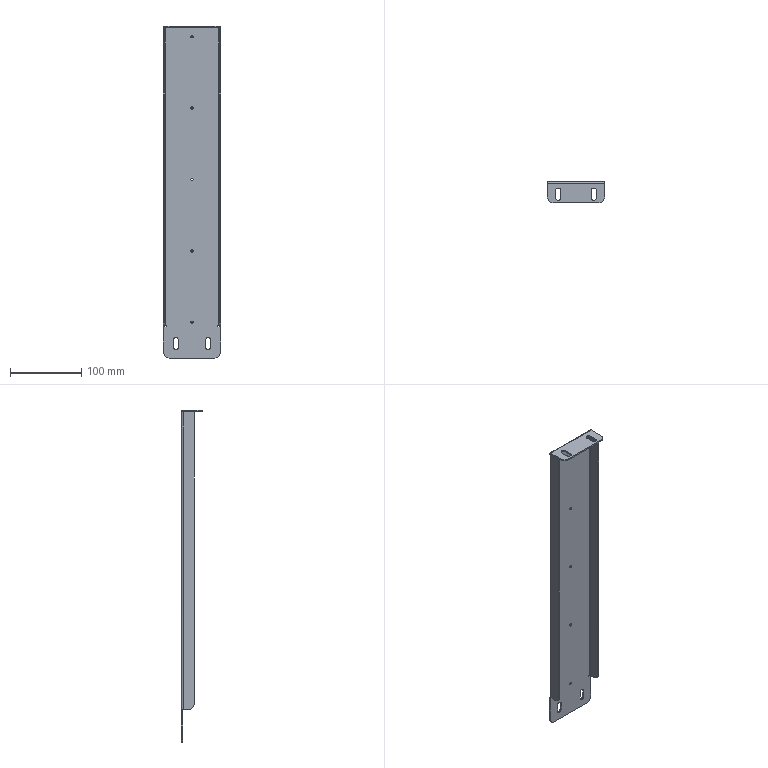Part | STEP file | TJ-DHQM-003-008 | 1 solid | 74 faces | box 80 x 30 x 465 mm | volume 103088 mm3 | plane 42 | cylinder 32 | commonest cylinder face diameters 3.3 x10 7 x10 16 x6 1.473 x3 5.473 x3